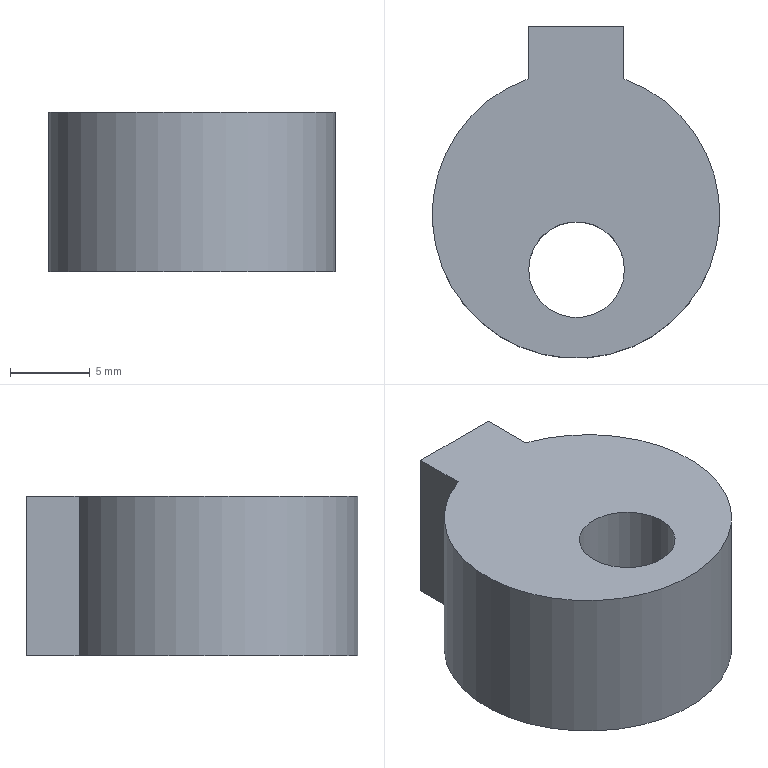CAM job | NX | 3-axis milling, drilling | part box 18 x 20.8 x 10 mm | stock box 40 x 70 x 10 mm
Tools:
number,name,description,diameter,corner_radius,flute_length,length,flutes
0,D6-18-D6-50-3T-FINISH,D6-18-D6-50-3T,6.0,0.0,18.0,50.0,3
0,钻头D4.0-54-83,钻刀D4.0-54-83,4.0,0.0,54.0,83.0,2
0,钻头D5.1-62-92,钻刀D5.1-62-92,5.1,0.0,62.0,92.0,2
0,上排M6-23-D6-63,上排M6-23-D6-63,6.0,0.0,23.0,26.0,2
0,倒角D8-90度,倒角D8-90度,8.0,0.0,8.0,60.0,2
Operations:
program,operation,operation_type,tool,method,geometry_group,spindle_rpm,surface_speed,feed_per_tooth,feed_cut,feed_plunge,cut_length_mm,path_length_mm,cut_time_min,machine_time_min
A1,DRILLING,Operation,倒角D8-90度,METHOD,WORKPIECE_54,2000.0,50.0,0.05,200.0,0.0,13.5,92.369,0.0675,0.0754
A1,DRILLING_COPY,Operation,钻头D4.0-54-83,METHOD,WORKPIECE_54,2000.0,50.0,0.05,200.0,0.0,32.0,113.708,0.16,0.1682
A1,DRILLING_COPY_1,Operation,钻头D5.1-62-92,METHOD,WORKPIECE_54,2000.0,50.0,0.05,200.0,0.0,23.0,86.0,0.115,0.1213
A1,DRILLING_COPY_1_COPY,Operation,上排M6-23-D6-63,METHOD,WORKPIECE_54,300.0,5.0,0.0017,1.0,0.0,8.0,56.0,8.0,8.005
A1,动态粗,CavityMilling,D6-18-D6-50-3T-FINISH,METHOD,WORKPIECE_54,4500.0,84.0,0.1481,2000.0,100.0,10888.732,10951.732,5.402,5.408
A1,PLANAR_MILL_COPY,PlanarMilling,倒角D8-90度,METHOD,WORKPIECE_54,3000.0,100.0,0.1178,600.0,100.0,82.608,121.608,0.1377,0.1416
A1,DRILLING_COPY_2,Operation,倒角D8-90度,METHOD,WORKPIECE_54,2000.0,50.0,0.05,200.0,0.0,6.2,52.4,0.031,0.0356
A1,PLANAR_MILL,PlanarMilling,D6-18-D6-50-3T-FINISH,METHOD,WORKPIECE_54,3000.0,100.0,0.1178,600.0,100.0,181.532,241.532,0.3026,0.3086